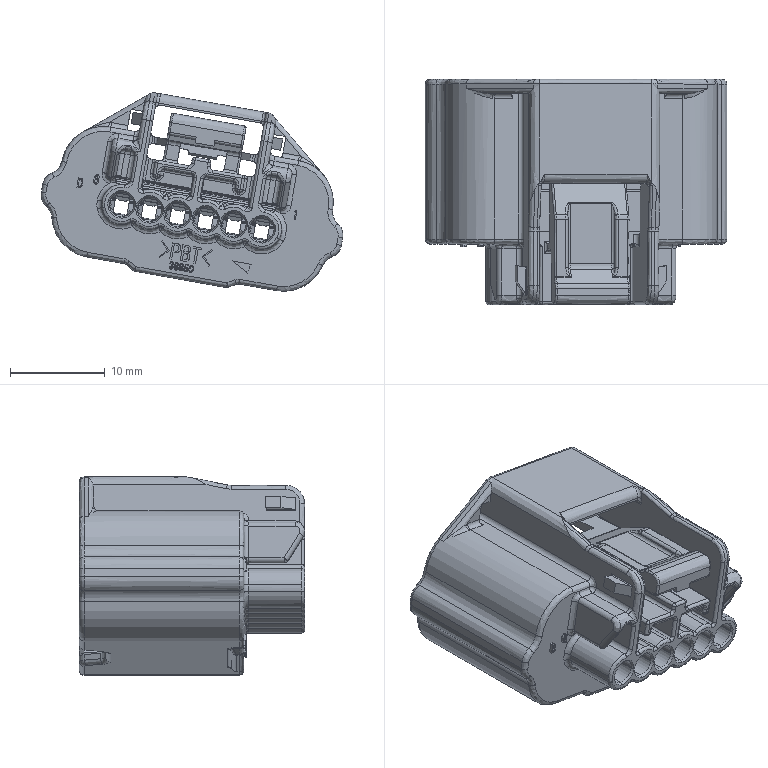Part | SolidWorks | features BaseBody 1 | 1 solid | 1682 faces | box 31.818 x 23.75 x 20.928 mm | volume 3737 mm3 | spline 679 | plane 647 | cylinder 295 | cone 36 | sphere 13 | torus 12 | commonest cylinder face diameters 0.6 x62 0.2 x55 1 x48 0.4 x34 2 x24 2.6 x24